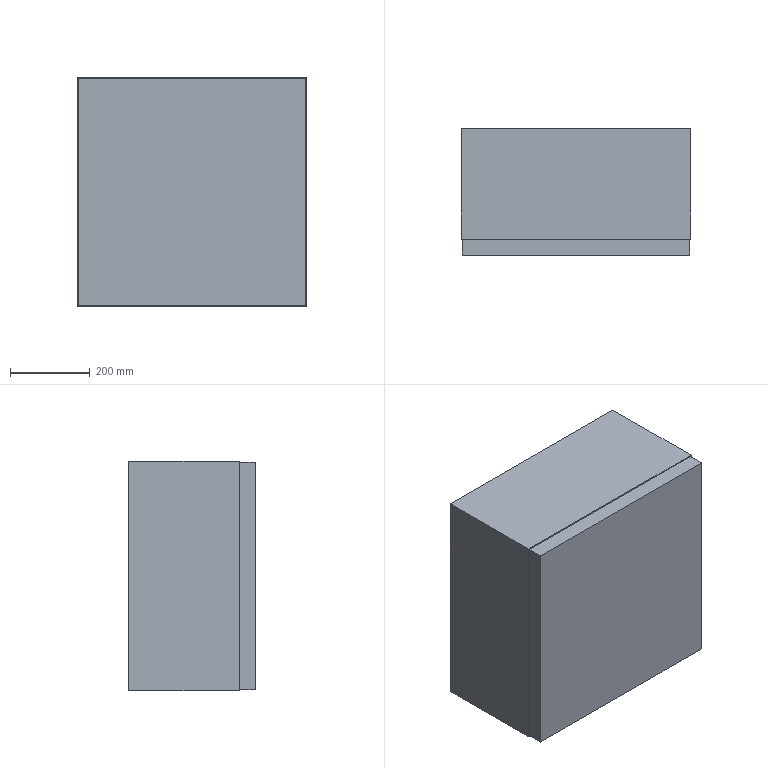Part | SolidWorks | features BaseBody 1 | 1 solid | 11 faces | box 575 x 317 x 575 mm | volume 104579125 mm3 | plane 11
STEP:
#1=CARTESIAN_POINT('',(285.,-40.,-285.));
#2=VERTEX_POINT('',#1);
#3=CARTESIAN_POINT('',(285.,-40.,285.));
#4=VERTEX_POINT('',#3);
#5=CARTESIAN_POINT('',(285.,-40.,-285.));
#6=DIRECTION('',(0.,0.,1.));
#7=VECTOR('',#6,1000.);
#8=LINE('',#5,#7);
#9=EDGE_CURVE('',#2,#4,#8,.T.);
#10=ORIENTED_EDGE('',*,*,#9,.T.);
#11=CARTESIAN_POINT('',(-285.,-40.,285.));
#12=VERTEX_POINT('',#11);
#13=CARTESIAN_POINT('',(-285.,-40.,285.));
#14=DIRECTION('',(-1.,0.,0.));
#15=VECTOR('',#14,1000.);
#16=LINE('',#13,#15);
#17=EDGE_CURVE('',#4,#12,#16,.T.);
#18=ORIENTED_EDGE('',*,*,#17,.T.);
#19=CARTESIAN_POINT('',(-285.,-40.,-285.));
#20=VERTEX_POINT('',#19);
#21=CARTESIAN_POINT('',(-285.,-40.,-285.));
#22=DIRECTION('',(0.,0.,-1.));
#23=VECTOR('',#22,1000.);
#24=LINE('',#21,#23);
#25=EDGE_CURVE('',#12,#20,#24,.T.);
#26=ORIENTED_EDGE('',*,*,#25,.T.);
#27=CARTESIAN_POINT('',(-285.,-40.,-285.));
#28=DIRECTION('',(1.,0.,0.));
#29=VECTOR('',#28,1000.);
#30=LINE('',#27,#29);
#31=EDGE_CURVE('',#20,#2,#30,.T.);
#32=ORIENTED_EDGE('',*,*,#31,.T.);
#33=EDGE_LOOP('',(#10,#18,#26,#32));
#34=FACE_OUTER_BOUND('',#33,.T.);
#35=CARTESIAN_POINT('',(0.,-40.,0.));
#36=DIRECTION('',(0.,1.,0.));
#37=DIRECTION('',(1.,0.,0.));
#38=AXIS2_PLACEMENT_3D('',#35,#36,#37);
#39=PLANE('',#38);
#40=ADVANCED_FACE('',(#34),#39,.F.);
#41=CARTESIAN_POINT('',(-285.,0.,-285.));
#42=VERTEX_POINT('',#41);
#43=CARTESIAN_POINT('',(285.,0.,-285.));
#44=VERTEX_POINT('',#43);
#45=CARTESIAN_POINT('',(-285.,0.,-285.));
#46=DIRECTION('',(1.,0.,0.));
#47=VECTOR('',#46,1000.);
#48=LINE('',#45,#47);
#49=EDGE_CURVE('',#42,#44,#48,.T.);
#50=ORIENTED_EDGE('',*,*,#49,.T.);
#51=CARTESIAN_POINT('',(285.,-40.,-285.));
#52=DIRECTION('',(0.,1.,0.));
#53=VECTOR('',#52,1000.);
#54=LINE('',#51,#53);
#55=EDGE_CURVE('',#2,#44,#54,.T.);
#56=ORIENTED_EDGE('',*,*,#55,.F.);
#57=ORIENTED_EDGE('',*,*,#31,.F.);
#58=CARTESIAN_POINT('',(-285.,-40.,-285.));
#59=DIRECTION('',(0.,1.,0.));
#60=VECTOR('',#59,1000.);
#61=LINE('',#58,#60);
#62=EDGE_CURVE('',#20,#42,#61,.T.);
#63=ORIENTED_EDGE('',*,*,#62,.T.);
#64=EDGE_LOOP('',(#50,#56,#57,#63));
#65=FACE_OUTER_BOUND('',#64,.T.);
#66=CARTESIAN_POINT('',(-285.,-40.,-285.));
#67=DIRECTION('',(0.,0.,1.));
#68=DIRECTION('',(1.,0.,0.));
#69=AXIS2_PLACEMENT_3D('',#66,#67,#68);
#70=PLANE('',#69);
#71=ADVANCED_FACE('',(#65),#70,.F.);
#72=CARTESIAN_POINT('',(-285.,0.,285.));
#73=VERTEX_POINT('',#72);
#74=CARTESIAN_POINT('',(-285.,0.,-285.));
#75=DIRECTION('',(0.,0.,-1.));
#76=VECTOR('',#75,1000.);
#77=LINE('',#74,#76);
#78=EDGE_CURVE('',#73,#42,#77,.T.);
#79=ORIENTED_EDGE('',*,*,#78,.T.);
#80=ORIENTED_EDGE('',*,*,#62,.F.);
#81=ORIENTED_EDGE('',*,*,#25,.F.);
#82=CARTESIAN_POINT('',(-285.,-40.,285.));
#83=DIRECTION('',(0.,1.,0.));
#84=VECTOR('',#83,1000.);
#85=LINE('',#82,#84);
#86=EDGE_CURVE('',#12,#73,#85,.T.);
#87=ORIENTED_EDGE('',*,*,#86,.T.);
#88=EDGE_LOOP('',(#79,#80,#81,#87));
#89=FACE_OUTER_BOUND('',#88,.T.);
#90=CARTESIAN_POINT('',(-285.,-40.,-285.));
#91=DIRECTION('',(1.,0.,0.));
#92=DIRECTION('',(0.,0.,1.));
#93=AXIS2_PLACEMENT_3D('',#90,#91,#92);
#94=PLANE('',#93);
#95=ADVANCED_FACE('',(#89),#94,.F.);
#96=CARTESIAN_POINT('',(285.,0.,285.));
#97=VERTEX_POINT('',#96);
#98=CARTESIAN_POINT('',(-285.,0.,285.));
#99=DIRECTION('',(-1.,0.,0.));
#100=VECTOR('',#99,1000.);
#101=LINE('',#98,#100);
#102=EDGE_CURVE('',#97,#73,#101,.T.);
#103=ORIENTED_EDGE('',*,*,#102,.T.);
#104=ORIENTED_EDGE('',*,*,#86,.F.);
#105=ORIENTED_EDGE('',*,*,#17,.F.);
#106=CARTESIAN_POINT('',(285.,-40.,285.));
#107=DIRECTION('',(0.,1.,0.));
#108=VECTOR('',#107,1000.);
#109=LINE('',#106,#108);
#110=EDGE_CURVE('',#4,#97,#109,.T.);
#111=ORIENTED_EDGE('',*,*,#110,.T.);
#112=EDGE_LOOP('',(#103,#104,#105,#111));
#113=FACE_OUTER_BOUND('',#112,.T.);
#114=CARTESIAN_POINT('',(-285.,-40.,285.));
#115=DIRECTION('',(0.,0.,-1.));
#116=DIRECTION('',(0.,-1.,0.));
#117=AXIS2_PLACEMENT_3D('',#114,#115,#116);
#118=PLANE('',#117);
#119=ADVANCED_FACE('',(#113),#118,.F.);
#120=CARTESIAN_POINT('',(285.,0.,-285.));
#121=DIRECTION('',(0.,0.,1.));
#122=VECTOR('',#121,1000.);
#123=LINE('',#120,#122);
#124=EDGE_CURVE('',#44,#97,#123,.T.);
#125=ORIENTED_EDGE('',*,*,#124,.T.);
#126=ORIENTED_EDGE('',*,*,#110,.F.);
#127=ORIENTED_EDGE('',*,*,#9,.F.);
#128=ORIENTED_EDGE('',*,*,#55,.T.);
#129=EDGE_LOOP('',(#125,#126,#127,#128));
#130=FACE_OUTER_BOUND('',#129,.T.);
#131=CARTESIAN_POINT('',(285.,-40.,-285.));
#132=DIRECTION('',(-1.,0.,0.));
#133=DIRECTION('',(0.,0.,1.));
#134=AXIS2_PLACEMENT_3D('',#131,#132,#133);
#135=PLANE('',#134);
#136=ADVANCED_FACE('',(#130),#135,.F.);
#137=CARTESIAN_POINT('',(287.5,277.,287.5));
#138=VERTEX_POINT('',#137);
#139=CARTESIAN_POINT('',(287.5,277.,-287.5));
#140=VERTEX_POINT('',#139);
#141=CARTESIAN_POINT('',(287.5,277.,287.5));
#142=DIRECTION('',(0.,0.,-1.));
#143=VECTOR('',#142,1000.);
#144=LINE('',#141,#143);
#145=EDGE_CURVE('',#138,#140,#144,.T.);
#146=ORIENTED_EDGE('',*,*,#145,.T.);
#147=CARTESIAN_POINT('',(-287.5,277.,-287.5));
#148=VERTEX_POINT('',#147);
#149=CARTESIAN_POINT('',(-287.5,277.,-287.5));
#150=DIRECTION('',(-1.,0.,0.));
#151=VECTOR('',#150,1000.);
#152=LINE('',#149,#151);
#153=EDGE_CURVE('',#140,#148,#152,.T.);
#154=ORIENTED_EDGE('',*,*,#153,.T.);
#155=CARTESIAN_POINT('',(-287.5,277.,287.5));
#156=VERTEX_POINT('',#155);
#157=CARTESIAN_POINT('',(-287.5,277.,287.5));
#158=DIRECTION('',(0.,0.,1.));
#159=VECTOR('',#158,1000.);
#160=LINE('',#157,#159);
#161=EDGE_CURVE('',#148,#156,#160,.T.);
#162=ORIENTED_EDGE('',*,*,#161,.T.);
#163=CARTESIAN_POINT('',(-287.5,277.,287.5));
#164=DIRECTION('',(1.,0.,0.));
#165=VECTOR('',#164,1000.);
#166=LINE('',#163,#165);
#167=EDGE_CURVE('',#156,#138,#166,.T.);
#168=ORIENTED_EDGE('',*,*,#167,.T.);
#169=EDGE_LOOP('',(#146,#154,#162,#168));
#170=FACE_OUTER_BOUND('',#169,.T.);
#171=CARTESIAN_POINT('',(0.,277.,0.));
#172=DIRECTION('',(0.,-1.,0.));
#173=DIRECTION('',(0.,0.,-1.));
#174=AXIS2_PLACEMENT_3D('',#171,#172,#173);
#175=PLANE('',#174);
#176=ADVANCED_FACE('',(#170),#175,.F.);
#177=CARTESIAN_POINT('',(-287.5,0.,287.5));
#178=VERTEX_POINT('',#177);
#179=CARTESIAN_POINT('',(287.5,0.,287.5));
#180=VERTEX_POINT('',#179);
#181=CARTESIAN_POINT('',(-287.5,0.,287.5));
#182=DIRECTION('',(1.,0.,0.));
#183=VECTOR('',#182,1000.);
#184=LINE('',#181,#183);
#185=EDGE_CURVE('',#178,#180,#184,.T.);
#186=ORIENTED_EDGE('',*,*,#185,.T.);
#187=CARTESIAN_POINT('',(287.5,277.,287.5));
#188=DIRECTION('',(0.,-1.,0.));
#189=VECTOR('',#188,1000.);
#190=LINE('',#187,#189);
#191=EDGE_CURVE('',#138,#180,#190,.T.);
#192=ORIENTED_EDGE('',*,*,#191,.F.);
#193=ORIENTED_EDGE('',*,*,#167,.F.);
#194=CARTESIAN_POINT('',(-287.5,277.,287.5));
#195=DIRECTION('',(0.,-1.,0.));
#196=VECTOR('',#195,1000.);
#197=LINE('',#194,#196);
#198=EDGE_CURVE('',#156,#178,#197,.T.);
#199=ORIENTED_EDGE('',*,*,#198,.T.);
#200=EDGE_LOOP('',(#186,#192,#193,#199));
#201=FACE_OUTER_BOUND('',#200,.T.);
#202=CARTESIAN_POINT('',(-287.5,277.,287.5));
#203=DIRECTION('',(0.,0.,-1.));
#204=DIRECTION('',(0.,-1.,0.));
#205=AXIS2_PLACEMENT_3D('',#202,#203,#204);
#206=PLANE('',#205);
#207=ADVANCED_FACE('',(#201),#206,.F.);
#208=CARTESIAN_POINT('',(-287.5,0.,-287.5));
#209=VERTEX_POINT('',#208);
#210=CARTESIAN_POINT('',(-287.5,0.,287.5));
#211=DIRECTION('',(0.,0.,1.));
#212=VECTOR('',#211,1000.);
#213=LINE('',#210,#212);
#214=EDGE_CURVE('',#209,#178,#213,.T.);
#215=ORIENTED_EDGE('',*,*,#214,.T.);
#216=ORIENTED_EDGE('',*,*,#198,.F.);
#217=ORIENTED_EDGE('',*,*,#161,.F.);
#218=CARTESIAN_POINT('',(-287.5,277.,-287.5));
#219=DIRECTION('',(0.,-1.,0.));
#220=VECTOR('',#219,1000.);
#221=LINE('',#218,#220);
#222=EDGE_CURVE('',#148,#209,#221,.T.);
#223=ORIENTED_EDGE('',*,*,#222,.T.);
#224=EDGE_LOOP('',(#215,#216,#217,#223));
#225=FACE_OUTER_BOUND('',#224,.T.);
#226=CARTESIAN_POINT('',(-287.5,277.,287.5));
#227=DIRECTION('',(1.,0.,0.));
#228=DIRECTION('',(0.,1.,0.));
#229=AXIS2_PLACEMENT_3D('',#226,#227,#228);
#230=PLANE('',#229);
#231=ADVANCED_FACE('',(#225),#230,.F.);
#232=CARTESIAN_POINT('',(287.5,0.,-287.5));
#233=VERTEX_POINT('',#232);
#234=CARTESIAN_POINT('',(-287.5,0.,-287.5));
#235=DIRECTION('',(-1.,0.,0.));
#236=VECTOR('',#235,1000.);
#237=LINE('',#234,#236);
#238=EDGE_CURVE('',#233,#209,#237,.T.);
#239=ORIENTED_EDGE('',*,*,#238,.T.);
#240=ORIENTED_EDGE('',*,*,#222,.F.);
#241=ORIENTED_EDGE('',*,*,#153,.F.);
#242=CARTESIAN_POINT('',(287.5,277.,-287.5));
#243=DIRECTION('',(0.,-1.,0.));
#244=VECTOR('',#243,1000.);
#245=LINE('',#242,#244);
#246=EDGE_CURVE('',#140,#233,#245,.T.);
#247=ORIENTED_EDGE('',*,*,#246,.T.);
#248=EDGE_LOOP('',(#239,#240,#241,#247));
#249=FACE_OUTER_BOUND('',#248,.T.);
#250=CARTESIAN_POINT('',(-287.5,277.,-287.5));
#251=DIRECTION('',(0.,0.,1.));
#252=DIRECTION('',(1.,0.,0.));
#253=AXIS2_PLACEMENT_3D('',#250,#251,#252);
#254=PLANE('',#253);
#255=ADVANCED_FACE('',(#249),#254,.F.);
#256=CARTESIAN_POINT('',(287.5,0.,287.5));
#257=DIRECTION('',(0.,0.,-1.));
#258=VECTOR('',#257,1000.);
#259=LINE('',#256,#258);
#260=EDGE_CURVE('',#180,#233,#259,.T.);
#261=ORIENTED_EDGE('',*,*,#260,.T.);
#262=ORIENTED_EDGE('',*,*,#246,.F.);
#263=ORIENTED_EDGE('',*,*,#145,.F.);
#264=ORIENTED_EDGE('',*,*,#191,.T.);
#265=EDGE_LOOP('',(#261,#262,#263,#264));
#266=FACE_OUTER_BOUND('',#265,.T.);
#267=CARTESIAN_POINT('',(287.5,277.,287.5));
#268=DIRECTION('',(-1.,0.,0.));
#269=DIRECTION('',(0.,0.,1.));
#270=AXIS2_PLACEMENT_3D('',#267,#268,#269);
#271=PLANE('',#270);
#272=ADVANCED_FACE('',(#266),#271,.F.);
#273=ORIENTED_EDGE('',*,*,#102,.F.);
#274=ORIENTED_EDGE('',*,*,#124,.F.);
#275=ORIENTED_EDGE('',*,*,#49,.F.);
#276=ORIENTED_EDGE('',*,*,#78,.F.);
#277=EDGE_LOOP('',(#273,#274,#275,#276));
#278=FACE_BOUND('',#277,.T.);
#279=ORIENTED_EDGE('',*,*,#260,.F.);
#280=ORIENTED_EDGE('',*,*,#185,.F.);
#281=ORIENTED_EDGE('',*,*,#214,.F.);
#282=ORIENTED_EDGE('',*,*,#238,.F.);
#283=EDGE_LOOP('',(#279,#280,#281,#282));
#284=FACE_OUTER_BOUND('',#283,.T.);
#285=CARTESIAN_POINT('',(0.,0.,0.));
#286=DIRECTION('',(0.,-1.,0.));
#287=DIRECTION('',(0.,0.,-1.));
#288=AXIS2_PLACEMENT_3D('',#285,#286,#287);
#289=PLANE('',#288);
#290=ADVANCED_FACE('',(#278,#284),#289,.T.);
#291=CLOSED_SHELL('',(#40,#71,#95,#119,#136,#176,#207,#231,#255,#272,#290));
#292=MANIFOLD_SOLID_BREP('',#291);
#293=CARTESIAN_POINT('',(0.,0.,0.));
#294=DIRECTION('',(0.,0.,1.));
#295=DIRECTION('',(1.,0.,0.));
#296=AXIS2_PLACEMENT_3D('',#293,#294,#295);
#297=(LENGTH_UNIT()NAMED_UNIT(*)SI_UNIT(.MILLI.,.METRE.));
#298=UNCERTAINTY_MEASURE_WITH_UNIT(LENGTH_MEASURE(0.00001),#297,'','');
#299=(NAMED_UNIT(*)PLANE_ANGLE_UNIT()SI_UNIT($,.RADIAN.));
#300=(NAMED_UNIT(*)SI_UNIT($,.STERADIAN.)SOLID_ANGLE_UNIT());
#301=(GEOMETRIC_REPRESENTATION_CONTEXT(3)GLOBAL_UNCERTAINTY_ASSIGNED_CONTEXT((#298))GLOBAL_UNIT_ASSIGNED_CONTEXT((#297,#299,#300))REPRESENTATION_CONTEXT('',''));
#302=ADVANCED_BREP_SHAPE_REPRESENTATION('',(#292,#296),#301);